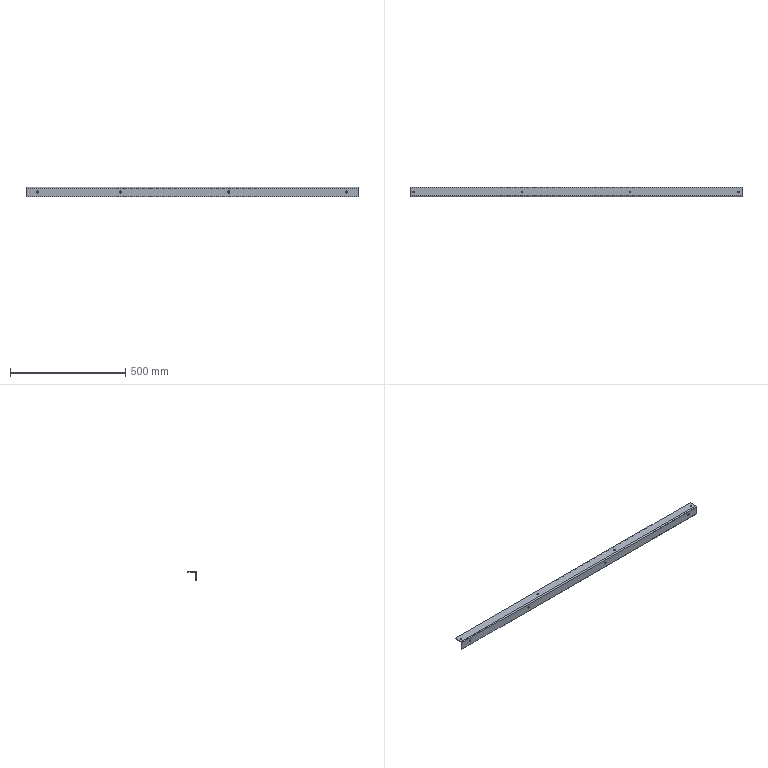Part | STEP file | 1 solid | 28 faces | box 1440 x 40 x 40 mm | volume 322453 mm3 | cylinder 20 | plane 8 | commonest cylinder face diameters 7 x8 9 x8 4 x3 10 x1